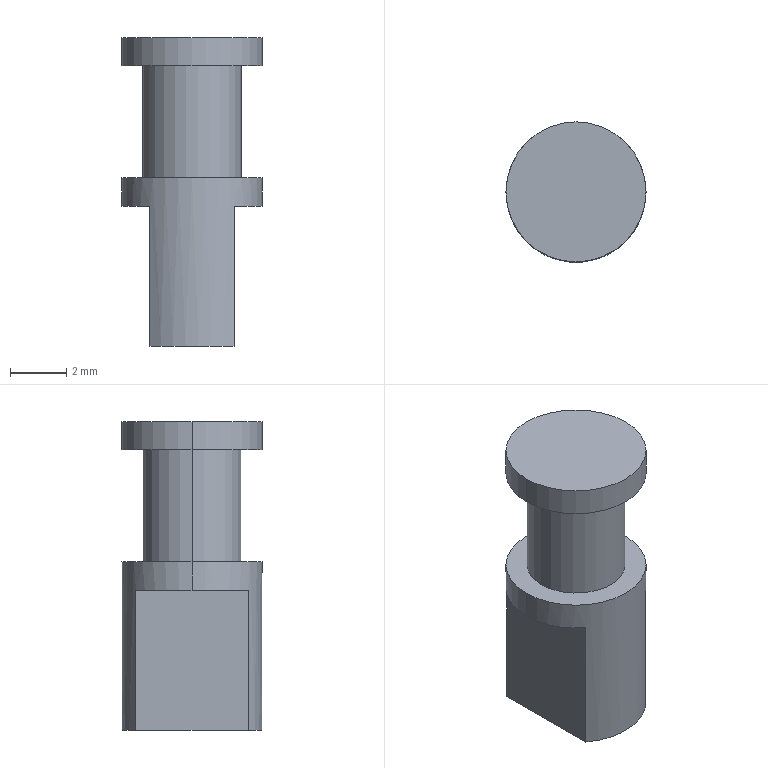Part | SolidWorks | features ICE 2, Attribute 1, Extrusion 1 | 1 solid | 14 faces | box 5 x 5 x 11 mm | volume 147.973 mm3 | plane 8 | cylinder 6 | commonest cylinder face diameters 5 x4 3.5 x2
STEP:
#1=CARTESIAN_POINT('',(2.5,0.,11.));
#2=VERTEX_POINT('',#1);
#3=CARTESIAN_POINT('',(-2.5,0.,11.));
#4=VERTEX_POINT('',#3);
#5=CARTESIAN_POINT('',(0.,0.,11.));
#6=DIRECTION('',(0.,0.,1.));
#7=DIRECTION('',(1.,0.,0.));
#8=AXIS2_PLACEMENT_3D('',#5,#6,#7);
#9=CIRCLE('',#8,2.5);
#10=EDGE_CURVE('',#2,#4,#9,.T.);
#11=ORIENTED_EDGE('',*,*,#10,.F.);
#12=CARTESIAN_POINT('',(2.5,0.,10.));
#13=VERTEX_POINT('',#12);
#14=CARTESIAN_POINT('',(2.5,0.,11.));
#15=DIRECTION('',(0.,0.,-1.));
#16=VECTOR('',#15,1000.);
#17=LINE('',#14,#16);
#18=EDGE_CURVE('',#2,#13,#17,.T.);
#19=ORIENTED_EDGE('',*,*,#18,.T.);
#20=CARTESIAN_POINT('',(-2.5,0.,10.));
#21=VERTEX_POINT('',#20);
#22=CARTESIAN_POINT('',(0.,0.,10.));
#23=DIRECTION('',(0.,0.,1.));
#24=DIRECTION('',(1.,0.,0.));
#25=AXIS2_PLACEMENT_3D('',#22,#23,#24);
#26=CIRCLE('',#25,2.5);
#27=EDGE_CURVE('',#13,#21,#26,.T.);
#28=ORIENTED_EDGE('',*,*,#27,.T.);
#29=CARTESIAN_POINT('',(-2.5,0.,11.));
#30=DIRECTION('',(0.,0.,-1.));
#31=VECTOR('',#30,1000.);
#32=LINE('',#29,#31);
#33=EDGE_CURVE('',#4,#21,#32,.T.);
#34=ORIENTED_EDGE('',*,*,#33,.F.);
#35=EDGE_LOOP('',(#11,#19,#28,#34));
#36=FACE_OUTER_BOUND('',#35,.T.);
#37=CARTESIAN_POINT('',(0.,0.,11.));
#38=DIRECTION('',(0.,0.,-1.));
#39=DIRECTION('',(-1.,0.,0.));
#40=AXIS2_PLACEMENT_3D('',#37,#38,#39);
#41=CYLINDRICAL_SURFACE('',#40,2.5);
#42=ADVANCED_FACE('',(#36),#41,.T.);
#43=CARTESIAN_POINT('',(1.75,0.,6.));
#44=VERTEX_POINT('',#43);
#45=CARTESIAN_POINT('',(-1.75,0.,6.));
#46=VERTEX_POINT('',#45);
#47=CARTESIAN_POINT('',(0.,0.,6.));
#48=DIRECTION('',(0.,0.,1.));
#49=DIRECTION('',(1.,0.,0.));
#50=AXIS2_PLACEMENT_3D('',#47,#48,#49);
#51=CIRCLE('',#50,1.75);
#52=EDGE_CURVE('',#44,#46,#51,.T.);
#53=ORIENTED_EDGE('',*,*,#52,.T.);
#54=CARTESIAN_POINT('',(-1.75,0.,10.));
#55=VERTEX_POINT('',#54);
#56=CARTESIAN_POINT('',(-1.75,0.,6.));
#57=DIRECTION('',(0.,0.,1.));
#58=VECTOR('',#57,1000.);
#59=LINE('',#56,#58);
#60=EDGE_CURVE('',#46,#55,#59,.T.);
#61=ORIENTED_EDGE('',*,*,#60,.T.);
#62=CARTESIAN_POINT('',(1.75,0.,10.));
#63=VERTEX_POINT('',#62);
#64=CARTESIAN_POINT('',(0.,0.,10.));
#65=DIRECTION('',(0.,0.,1.));
#66=DIRECTION('',(1.,0.,0.));
#67=AXIS2_PLACEMENT_3D('',#64,#65,#66);
#68=CIRCLE('',#67,1.75);
#69=EDGE_CURVE('',#63,#55,#68,.T.);
#70=ORIENTED_EDGE('',*,*,#69,.F.);
#71=CARTESIAN_POINT('',(1.75,0.,6.));
#72=DIRECTION('',(0.,0.,1.));
#73=VECTOR('',#72,1000.);
#74=LINE('',#71,#73);
#75=EDGE_CURVE('',#44,#63,#74,.T.);
#76=ORIENTED_EDGE('',*,*,#75,.F.);
#77=EDGE_LOOP('',(#53,#61,#70,#76));
#78=FACE_OUTER_BOUND('',#77,.T.);
#79=CARTESIAN_POINT('',(0.,0.,6.));
#80=DIRECTION('',(0.,0.,1.));
#81=DIRECTION('',(1.,0.,0.));
#82=AXIS2_PLACEMENT_3D('',#79,#80,#81);
#83=CYLINDRICAL_SURFACE('',#82,1.75);
#84=ADVANCED_FACE('',(#78),#83,.T.);
#85=CARTESIAN_POINT('',(2.5,0.,6.));
#86=VERTEX_POINT('',#85);
#87=CARTESIAN_POINT('',(-2.5,0.,6.));
#88=VERTEX_POINT('',#87);
#89=CARTESIAN_POINT('',(0.,0.,6.));
#90=DIRECTION('',(0.,0.,1.));
#91=DIRECTION('',(1.,0.,0.));
#92=AXIS2_PLACEMENT_3D('',#89,#90,#91);
#93=CIRCLE('',#92,2.5);
#94=EDGE_CURVE('',#86,#88,#93,.T.);
#95=ORIENTED_EDGE('',*,*,#94,.F.);
#96=CARTESIAN_POINT('',(2.5,0.,5.));
#97=VERTEX_POINT('',#96);
#98=CARTESIAN_POINT('',(2.5,0.,11.));
#99=DIRECTION('',(0.,0.,-1.));
#100=VECTOR('',#99,1000.);
#101=LINE('',#98,#100);
#102=EDGE_CURVE('',#86,#97,#101,.T.);
#103=ORIENTED_EDGE('',*,*,#102,.T.);
#104=CARTESIAN_POINT('',(1.5,2.,5.));
#105=VERTEX_POINT('',#104);
#106=CARTESIAN_POINT('',(0.,0.,5.));
#107=DIRECTION('',(0.,0.,-1.));
#108=DIRECTION('',(-1.,0.,0.));
#109=AXIS2_PLACEMENT_3D('',#106,#107,#108);
#110=CIRCLE('',#109,2.5);
#111=EDGE_CURVE('',#105,#97,#110,.T.);
#112=ORIENTED_EDGE('',*,*,#111,.F.);
#113=CARTESIAN_POINT('',(1.5,2.,0.));
#114=VERTEX_POINT('',#113);
#115=CARTESIAN_POINT('',(1.5,2.,5.));
#116=DIRECTION('',(0.,0.,-1.));
#117=VECTOR('',#116,1000.);
#118=LINE('',#115,#117);
#119=EDGE_CURVE('',#105,#114,#118,.T.);
#120=ORIENTED_EDGE('',*,*,#119,.T.);
#121=CARTESIAN_POINT('',(-1.5,2.,0.));
#122=VERTEX_POINT('',#121);
#123=CARTESIAN_POINT('',(0.,0.,0.));
#124=DIRECTION('',(0.,0.,1.));
#125=DIRECTION('',(1.,0.,0.));
#126=AXIS2_PLACEMENT_3D('',#123,#124,#125);
#127=CIRCLE('',#126,2.5);
#128=EDGE_CURVE('',#114,#122,#127,.T.);
#129=ORIENTED_EDGE('',*,*,#128,.T.);
#130=CARTESIAN_POINT('',(-1.5,2.,5.));
#131=VERTEX_POINT('',#130);
#132=CARTESIAN_POINT('',(-1.5,2.,5.));
#133=DIRECTION('',(0.,0.,-1.));
#134=VECTOR('',#133,1000.);
#135=LINE('',#132,#134);
#136=EDGE_CURVE('',#131,#122,#135,.T.);
#137=ORIENTED_EDGE('',*,*,#136,.F.);
#138=CARTESIAN_POINT('',(-2.5,0.,5.));
#139=VERTEX_POINT('',#138);
#140=CARTESIAN_POINT('',(0.,0.,5.));
#141=DIRECTION('',(0.,0.,-1.));
#142=DIRECTION('',(-1.,0.,0.));
#143=AXIS2_PLACEMENT_3D('',#140,#141,#142);
#144=CIRCLE('',#143,2.5);
#145=EDGE_CURVE('',#139,#131,#144,.T.);
#146=ORIENTED_EDGE('',*,*,#145,.F.);
#147=CARTESIAN_POINT('',(-2.5,0.,11.));
#148=DIRECTION('',(0.,0.,-1.));
#149=VECTOR('',#148,1000.);
#150=LINE('',#147,#149);
#151=EDGE_CURVE('',#88,#139,#150,.T.);
#152=ORIENTED_EDGE('',*,*,#151,.F.);
#153=EDGE_LOOP('',(#95,#103,#112,#120,#129,#137,#146,#152));
#154=FACE_OUTER_BOUND('',#153,.T.);
#155=CARTESIAN_POINT('',(0.,0.,11.));
#156=DIRECTION('',(0.,0.,-1.));
#157=DIRECTION('',(-1.,0.,0.));
#158=AXIS2_PLACEMENT_3D('',#155,#156,#157);
#159=CYLINDRICAL_SURFACE('',#158,2.5);
#160=ADVANCED_FACE('',(#154),#159,.T.);
#161=ORIENTED_EDGE('',*,*,#102,.F.);
#162=CARTESIAN_POINT('',(0.,0.,6.));
#163=DIRECTION('',(0.,0.,1.));
#164=DIRECTION('',(1.,0.,0.));
#165=AXIS2_PLACEMENT_3D('',#162,#163,#164);
#166=CIRCLE('',#165,2.5);
#167=EDGE_CURVE('',#88,#86,#166,.T.);
#168=ORIENTED_EDGE('',*,*,#167,.F.);
#169=ORIENTED_EDGE('',*,*,#151,.T.);
#170=CARTESIAN_POINT('',(-1.5,-2.,5.));
#171=VERTEX_POINT('',#170);
#172=CARTESIAN_POINT('',(0.,0.,5.));
#173=DIRECTION('',(0.,0.,-1.));
#174=DIRECTION('',(-1.,0.,0.));
#175=AXIS2_PLACEMENT_3D('',#172,#173,#174);
#176=CIRCLE('',#175,2.5);
#177=EDGE_CURVE('',#171,#139,#176,.T.);
#178=ORIENTED_EDGE('',*,*,#177,.F.);
#179=CARTESIAN_POINT('',(-1.5,-2.,0.));
#180=VERTEX_POINT('',#179);
#181=CARTESIAN_POINT('',(-1.5,-2.,5.));
#182=DIRECTION('',(0.,0.,-1.));
#183=VECTOR('',#182,1000.);
#184=LINE('',#181,#183);
#185=EDGE_CURVE('',#171,#180,#184,.T.);
#186=ORIENTED_EDGE('',*,*,#185,.T.);
#187=CARTESIAN_POINT('',(1.5,-2.,0.));
#188=VERTEX_POINT('',#187);
#189=CARTESIAN_POINT('',(0.,0.,0.));
#190=DIRECTION('',(0.,0.,1.));
#191=DIRECTION('',(1.,0.,0.));
#192=AXIS2_PLACEMENT_3D('',#189,#190,#191);
#193=CIRCLE('',#192,2.5);
#194=EDGE_CURVE('',#180,#188,#193,.T.);
#195=ORIENTED_EDGE('',*,*,#194,.T.);
#196=CARTESIAN_POINT('',(1.5,-2.,5.));
#197=VERTEX_POINT('',#196);
#198=CARTESIAN_POINT('',(1.5,-2.,5.));
#199=DIRECTION('',(0.,0.,-1.));
#200=VECTOR('',#199,1000.);
#201=LINE('',#198,#200);
#202=EDGE_CURVE('',#197,#188,#201,.T.);
#203=ORIENTED_EDGE('',*,*,#202,.F.);
#204=CARTESIAN_POINT('',(0.,0.,5.));
#205=DIRECTION('',(0.,0.,-1.));
#206=DIRECTION('',(-1.,0.,0.));
#207=AXIS2_PLACEMENT_3D('',#204,#205,#206);
#208=CIRCLE('',#207,2.5);
#209=EDGE_CURVE('',#97,#197,#208,.T.);
#210=ORIENTED_EDGE('',*,*,#209,.F.);
#211=EDGE_LOOP('',(#161,#168,#169,#178,#186,#195,#203,#210));
#212=FACE_OUTER_BOUND('',#211,.T.);
#213=CARTESIAN_POINT('',(0.,0.,11.));
#214=DIRECTION('',(0.,0.,-1.));
#215=DIRECTION('',(-1.,0.,0.));
#216=AXIS2_PLACEMENT_3D('',#213,#214,#215);
#217=CYLINDRICAL_SURFACE('',#216,2.5);
#218=ADVANCED_FACE('',(#212),#217,.T.);
#219=CARTESIAN_POINT('',(-1.5,2.,0.));
#220=DIRECTION('',(0.,1.,0.));
#221=VECTOR('',#220,1000.);
#222=LINE('',#219,#221);
#223=EDGE_CURVE('',#180,#122,#222,.T.);
#224=ORIENTED_EDGE('',*,*,#223,.T.);
#225=ORIENTED_EDGE('',*,*,#128,.F.);
#226=CARTESIAN_POINT('',(1.5,2.,0.));
#227=DIRECTION('',(0.,-1.,0.));
#228=VECTOR('',#227,1000.);
#229=LINE('',#226,#228);
#230=EDGE_CURVE('',#114,#188,#229,.T.);
#231=ORIENTED_EDGE('',*,*,#230,.T.);
#232=ORIENTED_EDGE('',*,*,#194,.F.);
#233=EDGE_LOOP('',(#224,#225,#231,#232));
#234=FACE_OUTER_BOUND('',#233,.T.);
#235=CARTESIAN_POINT('',(0.,0.,0.));
#236=DIRECTION('',(0.,0.,1.));
#237=DIRECTION('',(1.,0.,0.));
#238=AXIS2_PLACEMENT_3D('',#235,#236,#237);
#239=PLANE('',#238);
#240=ADVANCED_FACE('',(#234),#239,.F.);
#241=ORIENTED_EDGE('',*,*,#230,.F.);
#242=ORIENTED_EDGE('',*,*,#119,.F.);
#243=CARTESIAN_POINT('',(1.5,2.,5.));
#244=DIRECTION('',(0.,-1.,0.));
#245=VECTOR('',#244,1000.);
#246=LINE('',#243,#245);
#247=EDGE_CURVE('',#105,#197,#246,.T.);
#248=ORIENTED_EDGE('',*,*,#247,.T.);
#249=ORIENTED_EDGE('',*,*,#202,.T.);
#250=EDGE_LOOP('',(#241,#242,#248,#249));
#251=FACE_OUTER_BOUND('',#250,.T.);
#252=CARTESIAN_POINT('',(1.5,2.,5.));
#253=DIRECTION('',(1.,0.,0.));
#254=DIRECTION('',(0.,0.,-1.));
#255=AXIS2_PLACEMENT_3D('',#252,#253,#254);
#256=PLANE('',#255);
#257=ADVANCED_FACE('',(#251),#256,.T.);
#258=ORIENTED_EDGE('',*,*,#111,.T.);
#259=ORIENTED_EDGE('',*,*,#209,.T.);
#260=ORIENTED_EDGE('',*,*,#247,.F.);
#261=EDGE_LOOP('',(#258,#259,#260));
#262=FACE_OUTER_BOUND('',#261,.T.);
#263=CARTESIAN_POINT('',(0.,0.,5.));
#264=DIRECTION('',(0.,0.,-1.));
#265=DIRECTION('',(-1.,0.,0.));
#266=AXIS2_PLACEMENT_3D('',#263,#264,#265);
#267=PLANE('',#266);
#268=ADVANCED_FACE('',(#262),#267,.T.);
#269=ORIENTED_EDGE('',*,*,#177,.T.);
#270=ORIENTED_EDGE('',*,*,#145,.T.);
#271=CARTESIAN_POINT('',(-1.5,2.,5.));
#272=DIRECTION('',(0.,1.,0.));
#273=VECTOR('',#272,1000.);
#274=LINE('',#271,#273);
#275=EDGE_CURVE('',#171,#131,#274,.T.);
#276=ORIENTED_EDGE('',*,*,#275,.F.);
#277=EDGE_LOOP('',(#269,#270,#276));
#278=FACE_OUTER_BOUND('',#277,.T.);
#279=CARTESIAN_POINT('',(0.,0.,5.));
#280=DIRECTION('',(0.,0.,-1.));
#281=DIRECTION('',(-1.,0.,0.));
#282=AXIS2_PLACEMENT_3D('',#279,#280,#281);
#283=PLANE('',#282);
#284=ADVANCED_FACE('',(#278),#283,.T.);
#285=ORIENTED_EDGE('',*,*,#223,.F.);
#286=ORIENTED_EDGE('',*,*,#185,.F.);
#287=ORIENTED_EDGE('',*,*,#275,.T.);
#288=ORIENTED_EDGE('',*,*,#136,.T.);
#289=EDGE_LOOP('',(#285,#286,#287,#288));
#290=FACE_OUTER_BOUND('',#289,.T.);
#291=CARTESIAN_POINT('',(-1.5,2.,5.));
#292=DIRECTION('',(-1.,0.,0.));
#293=DIRECTION('',(0.,0.,1.));
#294=AXIS2_PLACEMENT_3D('',#291,#292,#293);
#295=PLANE('',#294);
#296=ADVANCED_FACE('',(#290),#295,.T.);
#297=ORIENTED_EDGE('',*,*,#52,.F.);
#298=CARTESIAN_POINT('',(0.,0.,6.));
#299=DIRECTION('',(0.,0.,1.));
#300=DIRECTION('',(1.,0.,0.));
#301=AXIS2_PLACEMENT_3D('',#298,#299,#300);
#302=CIRCLE('',#301,1.75);
#303=EDGE_CURVE('',#46,#44,#302,.T.);
#304=ORIENTED_EDGE('',*,*,#303,.F.);
#305=EDGE_LOOP('',(#297,#304));
#306=FACE_BOUND('',#305,.T.);
#307=ORIENTED_EDGE('',*,*,#167,.T.);
#308=ORIENTED_EDGE('',*,*,#94,.T.);
#309=EDGE_LOOP('',(#307,#308));
#310=FACE_OUTER_BOUND('',#309,.T.);
#311=CARTESIAN_POINT('',(0.,0.,6.));
#312=DIRECTION('',(0.,0.,1.));
#313=DIRECTION('',(1.,0.,0.));
#314=AXIS2_PLACEMENT_3D('',#311,#312,#313);
#315=PLANE('',#314);
#316=ADVANCED_FACE('',(#306,#310),#315,.T.);
#317=ORIENTED_EDGE('',*,*,#69,.T.);
#318=CARTESIAN_POINT('',(0.,0.,10.));
#319=DIRECTION('',(0.,0.,1.));
#320=DIRECTION('',(1.,0.,0.));
#321=AXIS2_PLACEMENT_3D('',#318,#319,#320);
#322=CIRCLE('',#321,1.75);
#323=EDGE_CURVE('',#55,#63,#322,.T.);
#324=ORIENTED_EDGE('',*,*,#323,.T.);
#325=EDGE_LOOP('',(#317,#324));
#326=FACE_BOUND('',#325,.T.);
#327=CARTESIAN_POINT('',(0.,0.,10.));
#328=DIRECTION('',(0.,0.,1.));
#329=DIRECTION('',(1.,0.,0.));
#330=AXIS2_PLACEMENT_3D('',#327,#328,#329);
#331=CIRCLE('',#330,2.5);
#332=EDGE_CURVE('',#21,#13,#331,.T.);
#333=ORIENTED_EDGE('',*,*,#332,.F.);
#334=ORIENTED_EDGE('',*,*,#27,.F.);
#335=EDGE_LOOP('',(#333,#334));
#336=FACE_OUTER_BOUND('',#335,.T.);
#337=CARTESIAN_POINT('',(0.,0.,10.));
#338=DIRECTION('',(0.,0.,1.));
#339=DIRECTION('',(1.,0.,0.));
#340=AXIS2_PLACEMENT_3D('',#337,#338,#339);
#341=PLANE('',#340);
#342=ADVANCED_FACE('',(#326,#336),#341,.F.);
#343=ORIENTED_EDGE('',*,*,#60,.F.);
#344=ORIENTED_EDGE('',*,*,#303,.T.);
#345=ORIENTED_EDGE('',*,*,#75,.T.);
#346=ORIENTED_EDGE('',*,*,#323,.F.);
#347=EDGE_LOOP('',(#343,#344,#345,#346));
#348=FACE_OUTER_BOUND('',#347,.T.);
#349=CARTESIAN_POINT('',(0.,0.,6.));
#350=DIRECTION('',(0.,0.,1.));
#351=DIRECTION('',(1.,0.,0.));
#352=AXIS2_PLACEMENT_3D('',#349,#350,#351);
#353=CYLINDRICAL_SURFACE('',#352,1.75);
#354=ADVANCED_FACE('',(#348),#353,.T.);
#355=CARTESIAN_POINT('',(0.,0.,11.));
#356=DIRECTION('',(0.,0.,1.));
#357=DIRECTION('',(1.,0.,0.));
#358=AXIS2_PLACEMENT_3D('',#355,#356,#357);
#359=CIRCLE('',#358,2.5);
#360=EDGE_CURVE('',#4,#2,#359,.T.);
#361=ORIENTED_EDGE('',*,*,#360,.T.);
#362=ORIENTED_EDGE('',*,*,#10,.T.);
#363=EDGE_LOOP('',(#361,#362));
#364=FACE_OUTER_BOUND('',#363,.T.);
#365=CARTESIAN_POINT('',(0.,0.,11.));
#366=DIRECTION('',(0.,0.,1.));
#367=DIRECTION('',(1.,0.,0.));
#368=AXIS2_PLACEMENT_3D('',#365,#366,#367);
#369=PLANE('',#368);
#370=ADVANCED_FACE('',(#364),#369,.T.);
#371=ORIENTED_EDGE('',*,*,#18,.F.);
#372=ORIENTED_EDGE('',*,*,#360,.F.);
#373=ORIENTED_EDGE('',*,*,#33,.T.);
#374=ORIENTED_EDGE('',*,*,#332,.T.);
#375=EDGE_LOOP('',(#371,#372,#373,#374));
#376=FACE_OUTER_BOUND('',#375,.T.);
#377=CARTESIAN_POINT('',(0.,0.,11.));
#378=DIRECTION('',(0.,0.,-1.));
#379=DIRECTION('',(-1.,0.,0.));
#380=AXIS2_PLACEMENT_3D('',#377,#378,#379);
#381=CYLINDRICAL_SURFACE('',#380,2.5);
#382=ADVANCED_FACE('',(#376),#381,.T.);
#383=CLOSED_SHELL('',(#42,#84,#160,#218,#240,#257,#268,#284,#296,#316,#342,#354,#370,#382));
#384=MANIFOLD_SOLID_BREP('',#383);
#385=CARTESIAN_POINT('',(0.,0.,0.));
#386=DIRECTION('',(0.,0.,1.));
#387=DIRECTION('',(1.,0.,0.));
#388=AXIS2_PLACEMENT_3D('',#385,#386,#387);
#389=(LENGTH_UNIT()NAMED_UNIT(*)SI_UNIT(.MILLI.,.METRE.));
#390=UNCERTAINTY_MEASURE_WITH_UNIT(LENGTH_MEASURE(0.00001),#389,'','');
#391=(NAMED_UNIT(*)PLANE_ANGLE_UNIT()SI_UNIT($,.RADIAN.));
#392=(NAMED_UNIT(*)SI_UNIT($,.STERADIAN.)SOLID_ANGLE_UNIT());
#393=(GEOMETRIC_REPRESENTATION_CONTEXT(3)GLOBAL_UNCERTAINTY_ASSIGNED_CONTEXT((#390))GLOBAL_UNIT_ASSIGNED_CONTEXT((#389,#391,#392))REPRESENTATION_CONTEXT('',''));
#394=ADVANCED_BREP_SHAPE_REPRESENTATION('',(#384,#388),#393);